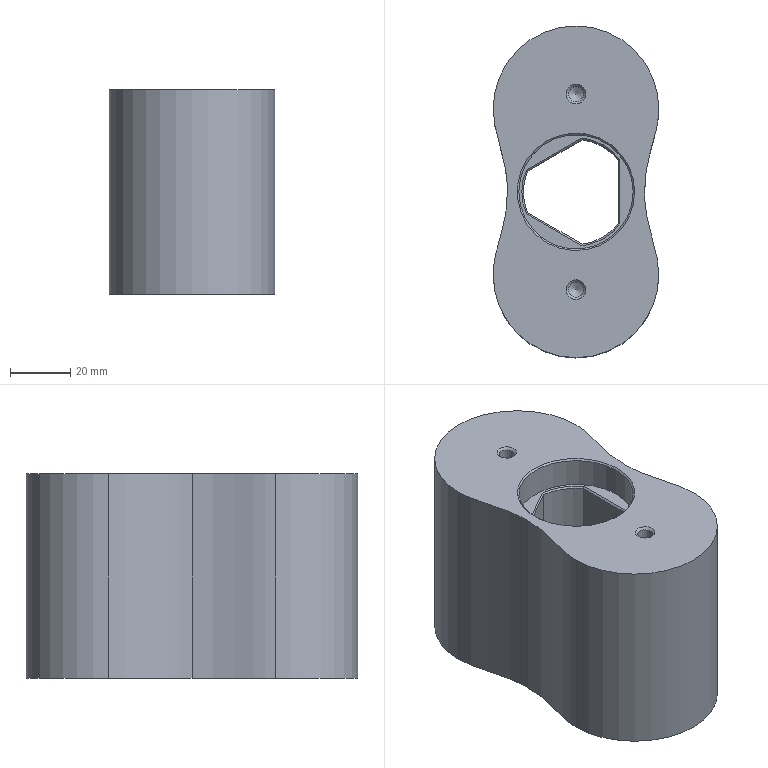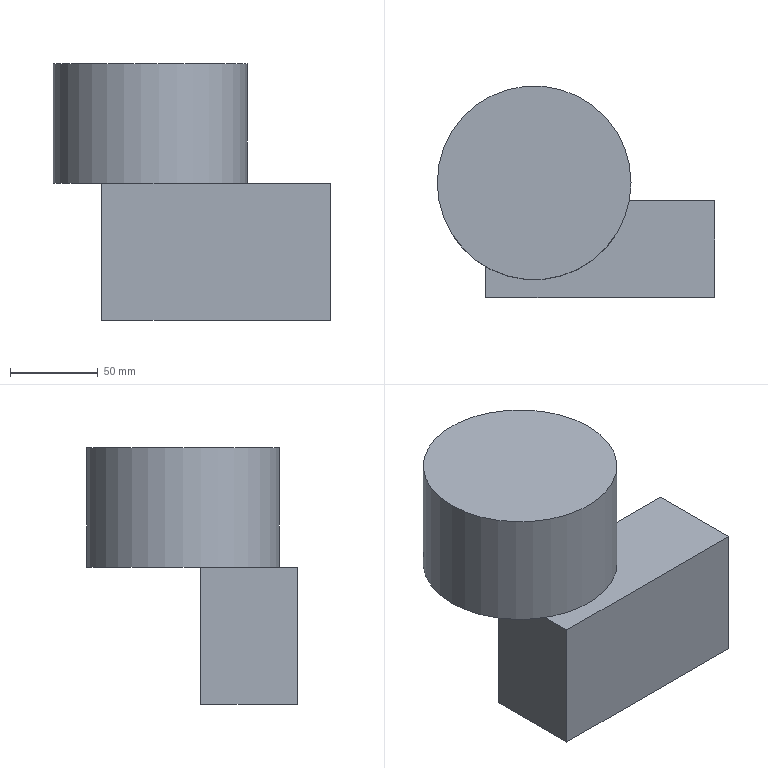CAM job | NX | 3-axis milling, drilling | part box 55.004 x 110.159 x 68 mm | stock box 157.736 x 120.159 x 146 mm
Tools:
number,name,description,diameter,corner_radius,flute_length,length,flutes
1,ZXZ,Milling Tool-5 Parameters,6.0,0.0,50.0,75.0,2
5,D25R0.5,Milling Tool-5 Parameters,25.0,0.5,50.0,75.0,2
12,D12,Milling Tool-5 Parameters,12.0,0.0,50.0,75.0,2
7,D6A45,Milling Tool-5 Parameters,6.0,0.0,50.0,75.0,2
12,2.5ZT,Drilling Tool,2.5,0.0,35.0,50.0,2
Operations:
program,operation,operation_type,tool,method,geometry_group,spindle_rpm,surface_speed,feed_per_tooth,feed_cut,feed_plunge,cut_length_mm,path_length_mm,cut_time_min,machine_time_min
1,DRILLING_COPY_1,Operation,ZXZ,METHOD,B,5000.0,94.0,0.025,250.0,0.0,8.0,119.611,0.032,0.0432
1,DRILLING_COPY_1_COPY,Operation,2.5ZT,METHOD,B,2000.0,15.0,0.03,120.0,0.0,21.502,146.615,0.1792,0.1917
1,ZLEVEL_PROFILE_COPY_1_COPY,ZLevelMilling,D12,METHOD,B,3000.0,113.0,0.3,1800.0,1000.0,17441.422,17558.222,9.744,9.756
1,CUTTERCOMP12_1_COPY,ZLevelMilling,D12,METHOD,B,5000.0,157.0,0.125,1250.0,100.0,4082.84,10515.222,3.266,3.909
2,ZLEVEL_PROFILE_COPY,ZLevelMilling,D25R0.5,METHOD,B,2000.0,157.0,0.55,2200.0,1000.0,35124.241,68098.32,17.399,32.254
2,ZLEVEL_PROFILE,ZLevelMilling,D25R0.5,METHOD,B,2000.0,157.0,0.55,2200.0,1000.0,71250.498,71372.498,32.456,32.469
2,CUTTERCOMP12,ZLevelMilling,D12,METHOD,B,5000.0,157.0,0.125,1250.0,100.0,22681.667,23092.166,18.145,18.186
2,PLANAR_MILL_COPY_COPY_COPY,PlanarMilling,D6A45,METHOD,B,7500.0,141.0,0.0833,1250.0,100.0,432.484,725.473,0.346,0.3753